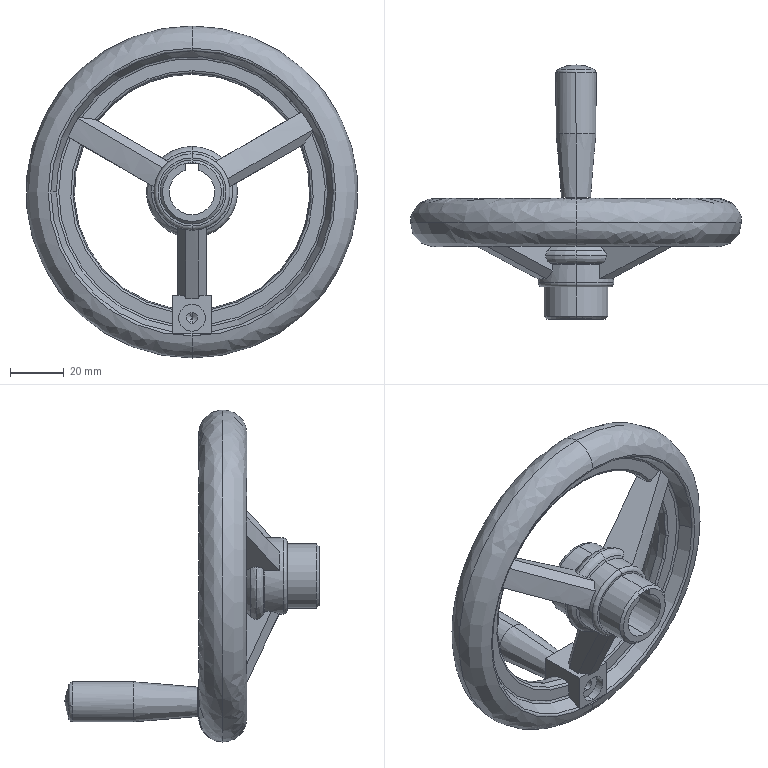Part | SolidWorks | features Draft 7, ICE 5, Fillet 4, BaseBody 1, Chamfer 1, HoleWzd 1, RevCut 1 | 1 solid | 178 faces | box 124 x 95 x 124 mm | volume 109982 mm3 | plane 72 | cylinder 43 | cone 30 | spline 22 | torus 11 | commonest cylinder face diameters 0.199 x8 28.472 x4 0.651 x3 0.637 x2 0.675 x2 0.729 x2